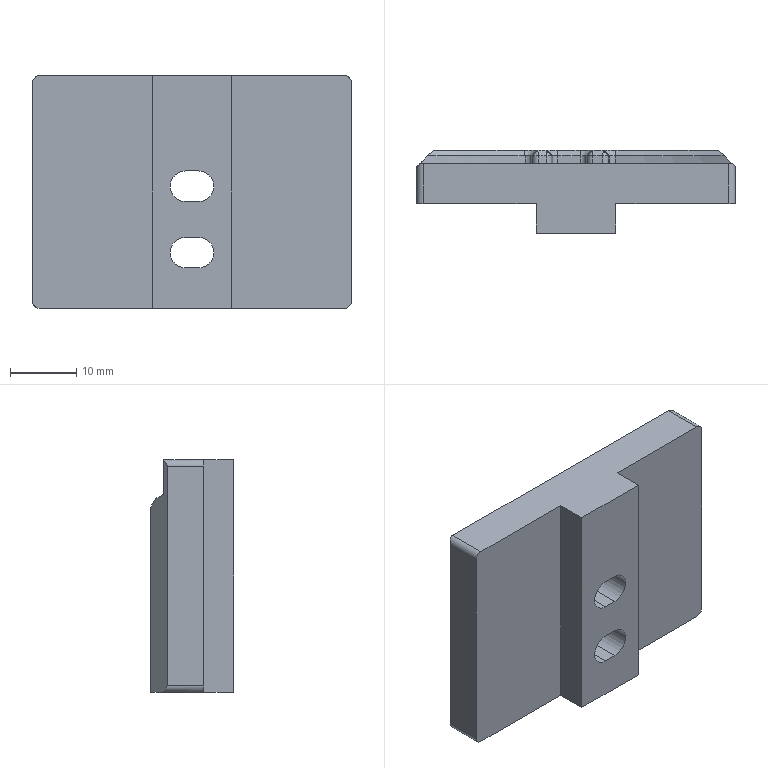Part | STEP file | product positioning block | 1 solid | 68 faces | box 48 x 12.5 x 35 mm | volume 13200 mm3 | plane 30 | cylinder 25 | cone 13 | commonest cylinder face diameters 1.6 x8 2 x4 4 x4 4.6 x4 96 x3 89 x2